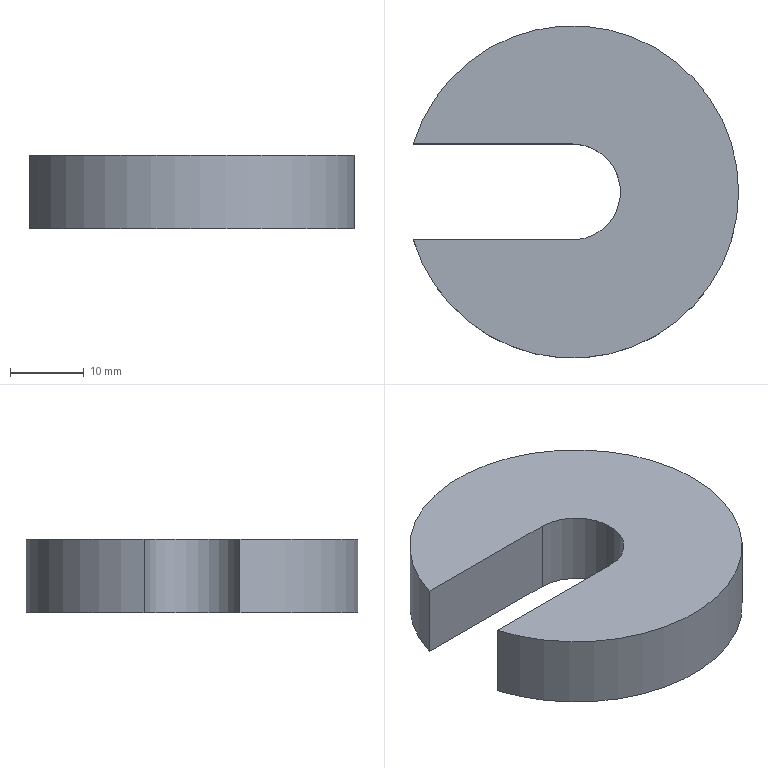Part | SolidWorks | features Extrusion 1 | 1 solid | 6 faces | box 44.041 x 45 x 10 mm | volume 12357 mm3 | plane 4 | cylinder 2 | commonest cylinder face diameters 13 x1 45 x1
STEP:
#1=CARTESIAN_POINT('',(0.,6.5,0.));
#2=VERTEX_POINT('',#1);
#3=CARTESIAN_POINT('',(0.,-6.5,0.));
#4=VERTEX_POINT('',#3);
#5=CARTESIAN_POINT('',(0.,0.,0.));
#6=DIRECTION('',(0.,0.,-1.));
#7=DIRECTION('',(1.,0.,0.));
#8=AXIS2_PLACEMENT_3D('',#5,#6,#7);
#9=CIRCLE('',#8,6.5);
#10=EDGE_CURVE('',#2,#4,#9,.T.);
#11=ORIENTED_EDGE('',*,*,#10,.T.);
#12=CARTESIAN_POINT('',(0.,-6.5,10.));
#13=VERTEX_POINT('',#12);
#14=CARTESIAN_POINT('',(0.,-6.5,10.));
#15=DIRECTION('',(0.,0.,-1.));
#16=VECTOR('',#15,1000.);
#17=LINE('',#14,#16);
#18=EDGE_CURVE('',#13,#4,#17,.T.);
#19=ORIENTED_EDGE('',*,*,#18,.F.);
#20=CARTESIAN_POINT('',(0.,6.5,10.));
#21=VERTEX_POINT('',#20);
#22=CARTESIAN_POINT('',(0.,0.,10.));
#23=DIRECTION('',(0.,0.,-1.));
#24=DIRECTION('',(1.,0.,0.));
#25=AXIS2_PLACEMENT_3D('',#22,#23,#24);
#26=CIRCLE('',#25,6.5);
#27=EDGE_CURVE('',#21,#13,#26,.T.);
#28=ORIENTED_EDGE('',*,*,#27,.F.);
#29=CARTESIAN_POINT('',(0.,6.5,10.));
#30=DIRECTION('',(0.,0.,-1.));
#31=VECTOR('',#30,1000.);
#32=LINE('',#29,#31);
#33=EDGE_CURVE('',#21,#2,#32,.T.);
#34=ORIENTED_EDGE('',*,*,#33,.T.);
#35=EDGE_LOOP('',(#11,#19,#28,#34));
#36=FACE_OUTER_BOUND('',#35,.T.);
#37=CARTESIAN_POINT('',(0.,0.,10.));
#38=DIRECTION('',(0.,0.,-1.));
#39=DIRECTION('',(-1.,0.,0.));
#40=AXIS2_PLACEMENT_3D('',#37,#38,#39);
#41=CYLINDRICAL_SURFACE('',#40,6.5);
#42=ADVANCED_FACE('',(#36),#41,.F.);
#43=CARTESIAN_POINT('',(-21.541,-6.5,0.));
#44=VERTEX_POINT('',#43);
#45=CARTESIAN_POINT('',(0.,-6.5,0.));
#46=DIRECTION('',(-1.,0.,0.));
#47=VECTOR('',#46,1000.);
#48=LINE('',#45,#47);
#49=EDGE_CURVE('',#4,#44,#48,.T.);
#50=ORIENTED_EDGE('',*,*,#49,.T.);
#51=CARTESIAN_POINT('',(-21.541,-6.5,10.));
#52=VERTEX_POINT('',#51);
#53=CARTESIAN_POINT('',(-21.541,-6.5,10.));
#54=DIRECTION('',(0.,0.,-1.));
#55=VECTOR('',#54,1000.);
#56=LINE('',#53,#55);
#57=EDGE_CURVE('',#52,#44,#56,.T.);
#58=ORIENTED_EDGE('',*,*,#57,.F.);
#59=CARTESIAN_POINT('',(0.,-6.5,10.));
#60=DIRECTION('',(-1.,0.,0.));
#61=VECTOR('',#60,1000.);
#62=LINE('',#59,#61);
#63=EDGE_CURVE('',#13,#52,#62,.T.);
#64=ORIENTED_EDGE('',*,*,#63,.F.);
#65=ORIENTED_EDGE('',*,*,#18,.T.);
#66=EDGE_LOOP('',(#50,#58,#64,#65));
#67=FACE_OUTER_BOUND('',#66,.T.);
#68=CARTESIAN_POINT('',(0.,-6.5,10.));
#69=DIRECTION('',(0.,-1.,0.));
#70=DIRECTION('',(0.,0.,-1.));
#71=AXIS2_PLACEMENT_3D('',#68,#69,#70);
#72=PLANE('',#71);
#73=ADVANCED_FACE('',(#67),#72,.F.);
#74=CARTESIAN_POINT('',(-21.541,6.5,0.));
#75=VERTEX_POINT('',#74);
#76=CARTESIAN_POINT('',(0.,0.,0.));
#77=DIRECTION('',(0.,0.,1.));
#78=DIRECTION('',(1.,0.,0.));
#79=AXIS2_PLACEMENT_3D('',#76,#77,#78);
#80=CIRCLE('',#79,22.5);
#81=EDGE_CURVE('',#44,#75,#80,.T.);
#82=ORIENTED_EDGE('',*,*,#81,.T.);
#83=CARTESIAN_POINT('',(-21.541,6.5,10.));
#84=VERTEX_POINT('',#83);
#85=CARTESIAN_POINT('',(-21.541,6.5,10.));
#86=DIRECTION('',(0.,0.,-1.));
#87=VECTOR('',#86,1000.);
#88=LINE('',#85,#87);
#89=EDGE_CURVE('',#84,#75,#88,.T.);
#90=ORIENTED_EDGE('',*,*,#89,.F.);
#91=CARTESIAN_POINT('',(0.,0.,10.));
#92=DIRECTION('',(0.,0.,1.));
#93=DIRECTION('',(1.,0.,0.));
#94=AXIS2_PLACEMENT_3D('',#91,#92,#93);
#95=CIRCLE('',#94,22.5);
#96=EDGE_CURVE('',#52,#84,#95,.T.);
#97=ORIENTED_EDGE('',*,*,#96,.F.);
#98=ORIENTED_EDGE('',*,*,#57,.T.);
#99=EDGE_LOOP('',(#82,#90,#97,#98));
#100=FACE_OUTER_BOUND('',#99,.T.);
#101=CARTESIAN_POINT('',(0.,0.,10.));
#102=DIRECTION('',(0.,0.,-1.));
#103=DIRECTION('',(-1.,0.,0.));
#104=AXIS2_PLACEMENT_3D('',#101,#102,#103);
#105=CYLINDRICAL_SURFACE('',#104,22.5);
#106=ADVANCED_FACE('',(#100),#105,.T.);
#107=CARTESIAN_POINT('',(0.,6.5,0.));
#108=DIRECTION('',(1.,0.,0.));
#109=VECTOR('',#108,1000.);
#110=LINE('',#107,#109);
#111=EDGE_CURVE('',#75,#2,#110,.T.);
#112=ORIENTED_EDGE('',*,*,#111,.T.);
#113=ORIENTED_EDGE('',*,*,#33,.F.);
#114=CARTESIAN_POINT('',(0.,6.5,10.));
#115=DIRECTION('',(1.,0.,0.));
#116=VECTOR('',#115,1000.);
#117=LINE('',#114,#116);
#118=EDGE_CURVE('',#84,#21,#117,.T.);
#119=ORIENTED_EDGE('',*,*,#118,.F.);
#120=ORIENTED_EDGE('',*,*,#89,.T.);
#121=EDGE_LOOP('',(#112,#113,#119,#120));
#122=FACE_OUTER_BOUND('',#121,.T.);
#123=CARTESIAN_POINT('',(0.,6.5,10.));
#124=DIRECTION('',(0.,1.,0.));
#125=DIRECTION('',(0.,0.,1.));
#126=AXIS2_PLACEMENT_3D('',#123,#124,#125);
#127=PLANE('',#126);
#128=ADVANCED_FACE('',(#122),#127,.F.);
#129=ORIENTED_EDGE('',*,*,#27,.T.);
#130=ORIENTED_EDGE('',*,*,#63,.T.);
#131=ORIENTED_EDGE('',*,*,#96,.T.);
#132=ORIENTED_EDGE('',*,*,#118,.T.);
#133=EDGE_LOOP('',(#129,#130,#131,#132));
#134=FACE_OUTER_BOUND('',#133,.T.);
#135=CARTESIAN_POINT('',(0.,0.,10.));
#136=DIRECTION('',(0.,0.,1.));
#137=DIRECTION('',(1.,0.,0.));
#138=AXIS2_PLACEMENT_3D('',#135,#136,#137);
#139=PLANE('',#138);
#140=ADVANCED_FACE('',(#134),#139,.T.);
#141=ORIENTED_EDGE('',*,*,#10,.F.);
#142=ORIENTED_EDGE('',*,*,#111,.F.);
#143=ORIENTED_EDGE('',*,*,#81,.F.);
#144=ORIENTED_EDGE('',*,*,#49,.F.);
#145=EDGE_LOOP('',(#141,#142,#143,#144));
#146=FACE_OUTER_BOUND('',#145,.T.);
#147=CARTESIAN_POINT('',(0.,0.,0.));
#148=DIRECTION('',(0.,0.,1.));
#149=DIRECTION('',(1.,0.,0.));
#150=AXIS2_PLACEMENT_3D('',#147,#148,#149);
#151=PLANE('',#150);
#152=ADVANCED_FACE('',(#146),#151,.F.);
#153=CLOSED_SHELL('',(#42,#73,#106,#128,#140,#152));
#154=MANIFOLD_SOLID_BREP('',#153);
#155=CARTESIAN_POINT('',(0.,0.,0.));
#156=DIRECTION('',(0.,0.,1.));
#157=DIRECTION('',(1.,0.,0.));
#158=AXIS2_PLACEMENT_3D('',#155,#156,#157);
#159=(LENGTH_UNIT()NAMED_UNIT(*)SI_UNIT(.MILLI.,.METRE.));
#160=UNCERTAINTY_MEASURE_WITH_UNIT(LENGTH_MEASURE(0.00001),#159,'','');
#161=(NAMED_UNIT(*)PLANE_ANGLE_UNIT()SI_UNIT($,.RADIAN.));
#162=(NAMED_UNIT(*)SI_UNIT($,.STERADIAN.)SOLID_ANGLE_UNIT());
#163=(GEOMETRIC_REPRESENTATION_CONTEXT(3)GLOBAL_UNCERTAINTY_ASSIGNED_CONTEXT((#160))GLOBAL_UNIT_ASSIGNED_CONTEXT((#159,#161,#162))REPRESENTATION_CONTEXT('',''));
#164=ADVANCED_BREP_SHAPE_REPRESENTATION('',(#154,#158),#163);